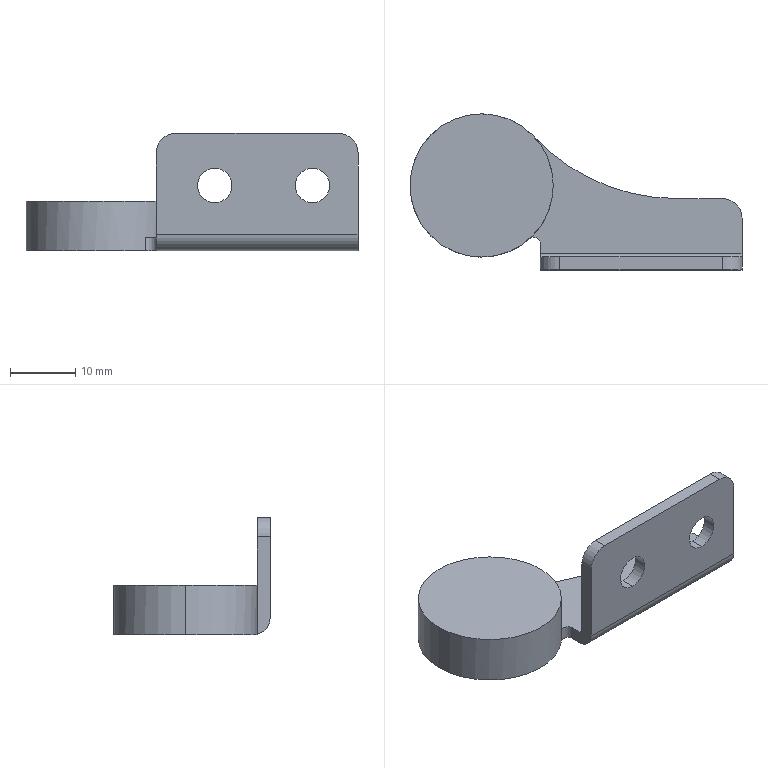Part | SolidWorks | features BaseBody 1 | 1 solid | 42 faces | box 51 x 24 x 18 mm | volume 4459 mm3 | cylinder 25 | plane 17 | commonest cylinder face diameters 0.528 x8 5.3 x4 6 x3 10 x2 10.02 x2 22 x2
STEP:
#1=CARTESIAN_POINT('',(-11.,0.,3.5));
#2=VERTEX_POINT('',#1);
#3=CARTESIAN_POINT('',(8.035,7.512,3.5));
#4=VERTEX_POINT('',#3);
#5=CARTESIAN_POINT('',(0.,0.,3.5));
#6=DIRECTION('',(0.,0.,-1.));
#7=DIRECTION('',(1.,0.,0.));
#8=AXIS2_PLACEMENT_3D('',#5,#6,#7);
#9=CIRCLE('',#8,11.);
#10=EDGE_CURVE('',#2,#4,#9,.T.);
#11=ORIENTED_EDGE('',*,*,#10,.F.);
#12=CARTESIAN_POINT('',(-11.,0.,11.1));
#13=VERTEX_POINT('',#12);
#14=CARTESIAN_POINT('',(-11.,0.,60.062));
#15=DIRECTION('',(0.,0.,1.));
#16=VECTOR('',#15,1000.);
#17=LINE('',#14,#16);
#18=EDGE_CURVE('',#2,#13,#17,.T.);
#19=ORIENTED_EDGE('',*,*,#18,.T.);
#20=CARTESIAN_POINT('',(11.,0.,11.1));
#21=VERTEX_POINT('',#20);
#22=CARTESIAN_POINT('',(0.,0.,11.1));
#23=DIRECTION('',(0.,0.,-1.));
#24=DIRECTION('',(1.,0.,0.));
#25=AXIS2_PLACEMENT_3D('',#22,#23,#24);
#26=CIRCLE('',#25,11.);
#27=EDGE_CURVE('',#13,#21,#26,.T.);
#28=ORIENTED_EDGE('',*,*,#27,.T.);
#29=CARTESIAN_POINT('',(11.,0.,5.5));
#30=VERTEX_POINT('',#29);
#31=CARTESIAN_POINT('',(11.,0.,60.062));
#32=DIRECTION('',(0.,0.,1.));
#33=VECTOR('',#32,1000.);
#34=LINE('',#31,#33);
#35=EDGE_CURVE('',#30,#21,#34,.T.);
#36=ORIENTED_EDGE('',*,*,#35,.F.);
#37=CARTESIAN_POINT('',(8.035,7.512,5.5));
#38=VERTEX_POINT('',#37);
#39=CARTESIAN_POINT('',(0.,0.,5.5));
#40=DIRECTION('',(0.,0.,1.));
#41=DIRECTION('',(1.,0.,0.));
#42=AXIS2_PLACEMENT_3D('',#39,#40,#41);
#43=CIRCLE('',#42,11.);
#44=EDGE_CURVE('',#30,#38,#43,.T.);
#45=ORIENTED_EDGE('',*,*,#44,.T.);
#46=CARTESIAN_POINT('',(8.035,7.512,3.5));
#47=DIRECTION('',(0.,0.,-1.));
#48=VECTOR('',#47,1000.);
#49=LINE('',#46,#48);
#50=EDGE_CURVE('',#38,#4,#49,.T.);
#51=ORIENTED_EDGE('',*,*,#50,.T.);
#52=EDGE_LOOP('',(#11,#19,#28,#36,#45,#51));
#53=FACE_OUTER_BOUND('',#52,.T.);
#54=CARTESIAN_POINT('',(0.,0.,60.062));
#55=DIRECTION('',(0.,0.,1.));
#56=DIRECTION('',(1.,0.,0.));
#57=AXIS2_PLACEMENT_3D('',#54,#55,#56);
#58=CYLINDRICAL_SURFACE('',#57,11.);
#59=ADVANCED_FACE('',(#53),#58,.T.);
#60=CARTESIAN_POINT('',(5.,0.,3.5));
#61=VERTEX_POINT('',#60);
#62=CARTESIAN_POINT('',(-5.,0.,3.5));
#63=VERTEX_POINT('',#62);
#64=CARTESIAN_POINT('',(0.,0.,3.5));
#65=DIRECTION('',(0.,0.,1.));
#66=DIRECTION('',(1.,0.,0.));
#67=AXIS2_PLACEMENT_3D('',#64,#65,#66);
#68=CIRCLE('',#67,5.);
#69=EDGE_CURVE('',#61,#63,#68,.T.);
#70=ORIENTED_EDGE('',*,*,#69,.T.);
#71=CARTESIAN_POINT('',(-5.,0.,5.5));
#72=VERTEX_POINT('',#71);
#73=CARTESIAN_POINT('',(-5.,0.,60.062));
#74=DIRECTION('',(0.,0.,1.));
#75=VECTOR('',#74,1000.);
#76=LINE('',#73,#75);
#77=EDGE_CURVE('',#63,#72,#76,.T.);
#78=ORIENTED_EDGE('',*,*,#77,.T.);
#79=CARTESIAN_POINT('',(5.,0.,5.5));
#80=VERTEX_POINT('',#79);
#81=CARTESIAN_POINT('',(0.,0.,5.5));
#82=DIRECTION('',(0.,0.,1.));
#83=DIRECTION('',(1.,0.,0.));
#84=AXIS2_PLACEMENT_3D('',#81,#82,#83);
#85=CIRCLE('',#84,5.);
#86=EDGE_CURVE('',#80,#72,#85,.T.);
#87=ORIENTED_EDGE('',*,*,#86,.F.);
#88=CARTESIAN_POINT('',(5.,0.,60.062));
#89=DIRECTION('',(0.,0.,1.));
#90=VECTOR('',#89,1000.);
#91=LINE('',#88,#90);
#92=EDGE_CURVE('',#61,#80,#91,.T.);
#93=ORIENTED_EDGE('',*,*,#92,.F.);
#94=EDGE_LOOP('',(#70,#78,#87,#93));
#95=FACE_OUTER_BOUND('',#94,.T.);
#96=CARTESIAN_POINT('',(0.,0.,60.062));
#97=DIRECTION('',(0.,0.,1.));
#98=DIRECTION('',(1.,0.,0.));
#99=AXIS2_PLACEMENT_3D('',#96,#97,#98);
#100=CYLINDRICAL_SURFACE('',#99,5.);
#101=ADVANCED_FACE('',(#95),#100,.T.);
#102=CARTESIAN_POINT('',(18.,-13.,16.15));
#103=VERTEX_POINT('',#102);
#104=CARTESIAN_POINT('',(18.,-13.,10.85));
#105=VERTEX_POINT('',#104);
#106=CARTESIAN_POINT('',(18.,-13.,13.5));
#107=DIRECTION('',(0.,-1.,0.));
#108=DIRECTION('',(0.,0.,1.));
#109=AXIS2_PLACEMENT_3D('',#106,#107,#108);
#110=CIRCLE('',#109,2.65);
#111=EDGE_CURVE('',#103,#105,#110,.T.);
#112=ORIENTED_EDGE('',*,*,#111,.T.);
#113=CARTESIAN_POINT('',(18.,-11.,10.85));
#114=VERTEX_POINT('',#113);
#115=CARTESIAN_POINT('',(18.,-13.,10.85));
#116=DIRECTION('',(0.,1.,0.));
#117=VECTOR('',#116,1000.);
#118=LINE('',#115,#117);
#119=EDGE_CURVE('',#105,#114,#118,.T.);
#120=ORIENTED_EDGE('',*,*,#119,.T.);
#121=CARTESIAN_POINT('',(18.,-11.,16.15));
#122=VERTEX_POINT('',#121);
#123=CARTESIAN_POINT('',(18.,-11.,13.5));
#124=DIRECTION('',(0.,-1.,0.));
#125=DIRECTION('',(0.,0.,1.));
#126=AXIS2_PLACEMENT_3D('',#123,#124,#125);
#127=CIRCLE('',#126,2.65);
#128=EDGE_CURVE('',#122,#114,#127,.T.);
#129=ORIENTED_EDGE('',*,*,#128,.F.);
#130=CARTESIAN_POINT('',(18.,-13.,16.15));
#131=DIRECTION('',(0.,1.,0.));
#132=VECTOR('',#131,1000.);
#133=LINE('',#130,#132);
#134=EDGE_CURVE('',#103,#122,#133,.T.);
#135=ORIENTED_EDGE('',*,*,#134,.F.);
#136=EDGE_LOOP('',(#112,#120,#129,#135));
#137=FACE_OUTER_BOUND('',#136,.T.);
#138=CARTESIAN_POINT('',(18.,-13.,13.5));
#139=DIRECTION('',(0.,1.,0.));
#140=DIRECTION('',(0.,0.,1.));
#141=AXIS2_PLACEMENT_3D('',#138,#139,#140);
#142=CYLINDRICAL_SURFACE('',#141,2.65);
#143=ADVANCED_FACE('',(#137),#142,.F.);
#144=CARTESIAN_POINT('',(33.,-13.,16.15));
#145=VERTEX_POINT('',#144);
#146=CARTESIAN_POINT('',(33.,-13.,10.85));
#147=VERTEX_POINT('',#146);
#148=CARTESIAN_POINT('',(33.,-13.,13.5));
#149=DIRECTION('',(0.,-1.,0.));
#150=DIRECTION('',(0.,0.,1.));
#151=AXIS2_PLACEMENT_3D('',#148,#149,#150);
#152=CIRCLE('',#151,2.65);
#153=EDGE_CURVE('',#145,#147,#152,.T.);
#154=ORIENTED_EDGE('',*,*,#153,.T.);
#155=CARTESIAN_POINT('',(33.,-11.,10.85));
#156=VERTEX_POINT('',#155);
#157=CARTESIAN_POINT('',(33.,-13.,10.85));
#158=DIRECTION('',(0.,1.,0.));
#159=VECTOR('',#158,1000.);
#160=LINE('',#157,#159);
#161=EDGE_CURVE('',#147,#156,#160,.T.);
#162=ORIENTED_EDGE('',*,*,#161,.T.);
#163=CARTESIAN_POINT('',(33.,-11.,16.15));
#164=VERTEX_POINT('',#163);
#165=CARTESIAN_POINT('',(33.,-11.,13.5));
#166=DIRECTION('',(0.,-1.,0.));
#167=DIRECTION('',(0.,0.,1.));
#168=AXIS2_PLACEMENT_3D('',#165,#166,#167);
#169=CIRCLE('',#168,2.65);
#170=EDGE_CURVE('',#164,#156,#169,.T.);
#171=ORIENTED_EDGE('',*,*,#170,.F.);
#172=CARTESIAN_POINT('',(33.,-13.,16.15));
#173=DIRECTION('',(0.,1.,0.));
#174=VECTOR('',#173,1000.);
#175=LINE('',#172,#174);
#176=EDGE_CURVE('',#145,#164,#175,.T.);
#177=ORIENTED_EDGE('',*,*,#176,.F.);
#178=EDGE_LOOP('',(#154,#162,#171,#177));
#179=FACE_OUTER_BOUND('',#178,.T.);
#180=CARTESIAN_POINT('',(33.,-13.,13.5));
#181=DIRECTION('',(0.,1.,0.));
#182=DIRECTION('',(0.,0.,1.));
#183=AXIS2_PLACEMENT_3D('',#180,#181,#182);
#184=CYLINDRICAL_SURFACE('',#183,2.65);
#185=ADVANCED_FACE('',(#179),#184,.F.);
#186=CARTESIAN_POINT('',(4.321,-2.76,3.5));
#187=VERTEX_POINT('',#186);
#188=CARTESIAN_POINT('',(4.105,-2.873,3.5));
#189=VERTEX_POINT('',#188);
#190=CARTESIAN_POINT('',(4.321,-3.024,3.5));
#191=DIRECTION('',(0.,0.,1.));
#192=DIRECTION('',(1.,0.,0.));
#193=AXIS2_PLACEMENT_3D('',#190,#191,#192);
#194=CIRCLE('',#193,0.264);
#195=EDGE_CURVE('',#187,#189,#194,.T.);
#196=ORIENTED_EDGE('',*,*,#195,.F.);
#197=CARTESIAN_POINT('',(6.436,-2.76,3.5));
#198=VERTEX_POINT('',#197);
#199=CARTESIAN_POINT('',(29.95,-2.76,3.5));
#200=DIRECTION('',(1.,0.,0.));
#201=VECTOR('',#200,1000.);
#202=LINE('',#199,#201);
#203=EDGE_CURVE('',#187,#198,#202,.T.);
#204=ORIENTED_EDGE('',*,*,#203,.T.);
#205=CARTESIAN_POINT('',(6.7,-2.496,3.5));
#206=VERTEX_POINT('',#205);
#207=CARTESIAN_POINT('',(6.436,-2.496,3.5));
#208=DIRECTION('',(0.,0.,1.));
#209=DIRECTION('',(1.,0.,0.));
#210=AXIS2_PLACEMENT_3D('',#207,#208,#209);
#211=CIRCLE('',#210,0.264);
#212=EDGE_CURVE('',#198,#206,#211,.T.);
#213=ORIENTED_EDGE('',*,*,#212,.T.);
#214=CARTESIAN_POINT('',(6.7,2.496,3.5));
#215=VERTEX_POINT('',#214);
#216=CARTESIAN_POINT('',(6.7,28.,3.5));
#217=DIRECTION('',(0.,1.,0.));
#218=VECTOR('',#217,1000.);
#219=LINE('',#216,#218);
#220=EDGE_CURVE('',#206,#215,#219,.T.);
#221=ORIENTED_EDGE('',*,*,#220,.T.);
#222=CARTESIAN_POINT('',(6.436,2.76,3.5));
#223=VERTEX_POINT('',#222);
#224=CARTESIAN_POINT('',(6.436,2.496,3.5));
#225=DIRECTION('',(0.,0.,1.));
#226=DIRECTION('',(1.,0.,0.));
#227=AXIS2_PLACEMENT_3D('',#224,#225,#226);
#228=CIRCLE('',#227,0.264);
#229=EDGE_CURVE('',#215,#223,#228,.T.);
#230=ORIENTED_EDGE('',*,*,#229,.T.);
#231=CARTESIAN_POINT('',(4.321,2.76,3.5));
#232=VERTEX_POINT('',#231);
#233=CARTESIAN_POINT('',(29.95,2.76,3.5));
#234=DIRECTION('',(-1.,0.,0.));
#235=VECTOR('',#234,1000.);
#236=LINE('',#233,#235);
#237=EDGE_CURVE('',#223,#232,#236,.T.);
#238=ORIENTED_EDGE('',*,*,#237,.T.);
#239=CARTESIAN_POINT('',(4.105,2.873,3.5));
#240=VERTEX_POINT('',#239);
#241=CARTESIAN_POINT('',(4.321,3.024,3.5));
#242=DIRECTION('',(0.,0.,1.));
#243=DIRECTION('',(1.,0.,0.));
#244=AXIS2_PLACEMENT_3D('',#241,#242,#243);
#245=CIRCLE('',#244,0.264);
#246=EDGE_CURVE('',#240,#232,#245,.T.);
#247=ORIENTED_EDGE('',*,*,#246,.F.);
#248=CARTESIAN_POINT('',(-4.105,2.873,3.5));
#249=VERTEX_POINT('',#248);
#250=CARTESIAN_POINT('',(0.,0.,3.5));
#251=DIRECTION('',(0.,0.,1.));
#252=DIRECTION('',(1.,0.,0.));
#253=AXIS2_PLACEMENT_3D('',#250,#251,#252);
#254=CIRCLE('',#253,5.01);
#255=EDGE_CURVE('',#240,#249,#254,.T.);
#256=ORIENTED_EDGE('',*,*,#255,.T.);
#257=CARTESIAN_POINT('',(-4.321,2.76,3.5));
#258=VERTEX_POINT('',#257);
#259=CARTESIAN_POINT('',(-4.321,3.024,3.5));
#260=DIRECTION('',(0.,0.,1.));
#261=DIRECTION('',(1.,0.,0.));
#262=AXIS2_PLACEMENT_3D('',#259,#260,#261);
#263=CIRCLE('',#262,0.264);
#264=EDGE_CURVE('',#258,#249,#263,.T.);
#265=ORIENTED_EDGE('',*,*,#264,.F.);
#266=CARTESIAN_POINT('',(-6.436,2.76,3.5));
#267=VERTEX_POINT('',#266);
#268=CARTESIAN_POINT('',(29.95,2.76,3.5));
#269=DIRECTION('',(-1.,0.,0.));
#270=VECTOR('',#269,1000.);
#271=LINE('',#268,#270);
#272=EDGE_CURVE('',#258,#267,#271,.T.);
#273=ORIENTED_EDGE('',*,*,#272,.T.);
#274=CARTESIAN_POINT('',(-6.7,2.496,3.5));
#275=VERTEX_POINT('',#274);
#276=CARTESIAN_POINT('',(-6.436,2.496,3.5));
#277=DIRECTION('',(0.,0.,1.));
#278=DIRECTION('',(1.,0.,0.));
#279=AXIS2_PLACEMENT_3D('',#276,#277,#278);
#280=CIRCLE('',#279,0.264);
#281=EDGE_CURVE('',#267,#275,#280,.T.);
#282=ORIENTED_EDGE('',*,*,#281,.T.);
#283=CARTESIAN_POINT('',(-6.7,-2.496,3.5));
#284=VERTEX_POINT('',#283);
#285=CARTESIAN_POINT('',(-6.7,28.,3.5));
#286=DIRECTION('',(0.,-1.,0.));
#287=VECTOR('',#286,1000.);
#288=LINE('',#285,#287);
#289=EDGE_CURVE('',#275,#284,#288,.T.);
#290=ORIENTED_EDGE('',*,*,#289,.T.);
#291=CARTESIAN_POINT('',(-6.436,-2.76,3.5));
#292=VERTEX_POINT('',#291);
#293=CARTESIAN_POINT('',(-6.436,-2.496,3.5));
#294=DIRECTION('',(0.,0.,1.));
#295=DIRECTION('',(1.,0.,0.));
#296=AXIS2_PLACEMENT_3D('',#293,#294,#295);
#297=CIRCLE('',#296,0.264);
#298=EDGE_CURVE('',#284,#292,#297,.T.);
#299=ORIENTED_EDGE('',*,*,#298,.T.);
#300=CARTESIAN_POINT('',(-4.321,-2.76,3.5));
#301=VERTEX_POINT('',#300);
#302=CARTESIAN_POINT('',(29.95,-2.76,3.5));
#303=DIRECTION('',(1.,0.,0.));
#304=VECTOR('',#303,1000.);
#305=LINE('',#302,#304);
#306=EDGE_CURVE('',#292,#301,#305,.T.);
#307=ORIENTED_EDGE('',*,*,#306,.T.);
#308=CARTESIAN_POINT('',(-4.105,-2.873,3.5));
#309=VERTEX_POINT('',#308);
#310=CARTESIAN_POINT('',(-4.321,-3.024,3.5));
#311=DIRECTION('',(0.,0.,1.));
#312=DIRECTION('',(1.,0.,0.));
#313=AXIS2_PLACEMENT_3D('',#310,#311,#312);
#314=CIRCLE('',#313,0.264);
#315=EDGE_CURVE('',#309,#301,#314,.T.);
#316=ORIENTED_EDGE('',*,*,#315,.F.);
#317=CARTESIAN_POINT('',(0.,0.,3.5));
#318=DIRECTION('',(0.,0.,1.));
#319=DIRECTION('',(1.,0.,0.));
#320=AXIS2_PLACEMENT_3D('',#317,#318,#319);
#321=CIRCLE('',#320,5.01);
#322=EDGE_CURVE('',#309,#189,#321,.T.);
#323=ORIENTED_EDGE('',*,*,#322,.T.);
#324=EDGE_LOOP('',(#196,#204,#213,#221,#230,#238,#247,#256,#265,#273,#282,#290,#299,#307,#316,#323));
#325=FACE_BOUND('',#324,.T.);
#326=CARTESIAN_POINT('',(29.95,-2.,3.5));
#327=VERTEX_POINT('',#326);
#328=CARTESIAN_POINT('',(37.,-2.,3.5));
#329=VERTEX_POINT('',#328);
#330=CARTESIAN_POINT('',(29.95,-2.,3.5));
#331=DIRECTION('',(1.,0.,0.));
#332=VECTOR('',#331,1000.);
#333=LINE('',#330,#332);
#334=EDGE_CURVE('',#327,#329,#333,.T.);
#335=ORIENTED_EDGE('',*,*,#334,.T.);
#336=CARTESIAN_POINT('',(40.,-5.,3.5));
#337=VERTEX_POINT('',#336);
#338=CARTESIAN_POINT('',(37.,-5.,3.5));
#339=DIRECTION('',(0.,0.,-1.));
#340=DIRECTION('',(1.,0.,0.));
#341=AXIS2_PLACEMENT_3D('',#338,#339,#340);
#342=CIRCLE('',#341,3.);
#343=EDGE_CURVE('',#329,#337,#342,.T.);
#344=ORIENTED_EDGE('',*,*,#343,.T.);
#345=CARTESIAN_POINT('',(40.,-10.5,3.5));
#346=VERTEX_POINT('',#345);
#347=CARTESIAN_POINT('',(40.,28.,3.5));
#348=DIRECTION('',(0.,-1.,0.));
#349=VECTOR('',#348,1000.);
#350=LINE('',#347,#349);
#351=EDGE_CURVE('',#337,#346,#350,.T.);
#352=ORIENTED_EDGE('',*,*,#351,.T.);
#353=CARTESIAN_POINT('',(9.,-10.5,3.5));
#354=VERTEX_POINT('',#353);
#355=CARTESIAN_POINT('',(29.95,-10.5,3.5));
#356=DIRECTION('',(-1.,0.,0.));
#357=VECTOR('',#356,1000.);
#358=LINE('',#355,#357);
#359=EDGE_CURVE('',#346,#354,#358,.T.);
#360=ORIENTED_EDGE('',*,*,#359,.T.);
#361=CARTESIAN_POINT('',(9.,-8.944,3.5));
#362=VERTEX_POINT('',#361);
#363=CARTESIAN_POINT('',(9.,-13.,3.5));
#364=DIRECTION('',(0.,-1.,0.));
#365=VECTOR('',#364,1000.);
#366=LINE('',#363,#365);
#367=EDGE_CURVE('',#362,#354,#366,.T.);
#368=ORIENTED_EDGE('',*,*,#367,.F.);
#369=CARTESIAN_POINT('',(7.333,-8.199,3.5));
#370=VERTEX_POINT('',#369);
#371=CARTESIAN_POINT('',(8.,-8.944,3.5));
#372=DIRECTION('',(0.,0.,1.));
#373=DIRECTION('',(1.,0.,0.));
#374=AXIS2_PLACEMENT_3D('',#371,#372,#373);
#375=CIRCLE('',#374,1.);
#376=EDGE_CURVE('',#362,#370,#375,.T.);
#377=ORIENTED_EDGE('',*,*,#376,.T.);
#378=CARTESIAN_POINT('',(0.,0.,3.5));
#379=DIRECTION('',(0.,0.,-1.));
#380=DIRECTION('',(1.,0.,0.));
#381=AXIS2_PLACEMENT_3D('',#378,#379,#380);
#382=CIRCLE('',#381,11.);
#383=EDGE_CURVE('',#370,#2,#382,.T.);
#384=ORIENTED_EDGE('',*,*,#383,.T.);
#385=ORIENTED_EDGE('',*,*,#10,.T.);
#386=CARTESIAN_POINT('',(29.95,28.,3.5));
#387=DIRECTION('',(0.,0.,1.));
#388=DIRECTION('',(1.,0.,0.));
#389=AXIS2_PLACEMENT_3D('',#386,#387,#388);
#390=CIRCLE('',#389,30.);
#391=EDGE_CURVE('',#4,#327,#390,.T.);
#392=ORIENTED_EDGE('',*,*,#391,.T.);
#393=EDGE_LOOP('',(#335,#344,#352,#360,#368,#377,#384,#385,#392));
#394=FACE_OUTER_BOUND('',#393,.T.);
#395=CARTESIAN_POINT('',(29.95,28.,3.5));
#396=DIRECTION('',(0.,0.,-1.));
#397=DIRECTION('',(-1.,0.,0.));
#398=AXIS2_PLACEMENT_3D('',#395,#396,#397);
#399=PLANE('',#398);
#400=ADVANCED_FACE('',(#325,#394),#399,.T.);
#401=CARTESIAN_POINT('',(6.436,-2.76,5.5));
#402=VERTEX_POINT('',#401);
#403=CARTESIAN_POINT('',(6.436,-2.76,3.5));
#404=DIRECTION('',(0.,0.,1.));
#405=VECTOR('',#404,1000.);
#406=LINE('',#403,#405);
#407=EDGE_CURVE('',#198,#402,#406,.T.);
#408=ORIENTED_EDGE('',*,*,#407,.F.);
#409=ORIENTED_EDGE('',*,*,#203,.F.);
#410=CARTESIAN_POINT('',(4.321,-2.76,5.5));
#411=VERTEX_POINT('',#410);
#412=CARTESIAN_POINT('',(4.321,-2.76,3.5));
#413=DIRECTION('',(0.,0.,-1.));
#414=VECTOR('',#413,1000.);
#415=LINE('',#412,#414);
#416=EDGE_CURVE('',#411,#187,#415,.T.);
#417=ORIENTED_EDGE('',*,*,#416,.F.);
#418=CARTESIAN_POINT('',(4.321,-2.76,5.5));
#419=DIRECTION('',(-1.,0.,0.));
#420=VECTOR('',#419,1000.);
#421=LINE('',#418,#420);
#422=EDGE_CURVE('',#402,#411,#421,.T.);
#423=ORIENTED_EDGE('',*,*,#422,.F.);
#424=EDGE_LOOP('',(#408,#409,#417,#423));
#425=FACE_OUTER_BOUND('',#424,.T.);
#426=CARTESIAN_POINT('',(4.321,-2.76,3.5));
#427=DIRECTION('',(0.,-1.,0.));
#428=DIRECTION('',(0.,0.,-1.));
#429=AXIS2_PLACEMENT_3D('',#426,#427,#428);
#430=PLANE('',#429);
#431=ADVANCED_FACE('',(#425),#430,.F.);
#432=CARTESIAN_POINT('',(4.105,-2.873,5.5));
#433=VERTEX_POINT('',#432);
#434=CARTESIAN_POINT('',(4.105,-2.873,3.5));
#435=DIRECTION('',(0.,0.,1.));
#436=VECTOR('',#435,1000.);
#437=LINE('',#434,#436);
#438=EDGE_CURVE('',#189,#433,#437,.T.);
#439=ORIENTED_EDGE('',*,*,#438,.F.);
#440=ORIENTED_EDGE('',*,*,#322,.F.);
#441=CARTESIAN_POINT('',(-4.105,-2.873,5.5));
#442=VERTEX_POINT('',#441);
#443=CARTESIAN_POINT('',(-4.105,-2.873,3.5));
#444=DIRECTION('',(0.,0.,-1.));
#445=VECTOR('',#444,1000.);
#446=LINE('',#443,#445);
#447=EDGE_CURVE('',#442,#309,#446,.T.);
#448=ORIENTED_EDGE('',*,*,#447,.F.);
#449=CARTESIAN_POINT('',(0.,0.,5.5));
#450=DIRECTION('',(0.,0.,-1.));
#451=DIRECTION('',(1.,0.,0.));
#452=AXIS2_PLACEMENT_3D('',#449,#450,#451);
#453=CIRCLE('',#452,5.01);
#454=EDGE_CURVE('',#433,#442,#453,.T.);
#455=ORIENTED_EDGE('',*,*,#454,.F.);
#456=EDGE_LOOP('',(#439,#440,#448,#455));
#457=FACE_OUTER_BOUND('',#456,.T.);
#458=CARTESIAN_POINT('',(0.,0.,3.5));
#459=DIRECTION('',(0.,0.,1.));
#460=DIRECTION('',(1.,0.,0.));
#461=AXIS2_PLACEMENT_3D('',#458,#459,#460);
#462=CYLINDRICAL_SURFACE('',#461,5.01);
#463=ADVANCED_FACE('',(#457),#462,.F.);
#464=CARTESIAN_POINT('',(-4.321,-2.76,5.5));
#465=VERTEX_POINT('',#464);
#466=CARTESIAN_POINT('',(-4.321,-2.76,3.5));
#467=DIRECTION('',(0.,0.,1.));
#468=VECTOR('',#467,1000.);
#469=LINE('',#466,#468);
#470=EDGE_CURVE('',#301,#465,#469,.T.);
#471=ORIENTED_EDGE('',*,*,#470,.F.);
#472=ORIENTED_EDGE('',*,*,#306,.F.);
#473=CARTESIAN_POINT('',(-6.436,-2.76,5.5));
#474=VERTEX_POINT('',#473);
#475=CARTESIAN_POINT('',(-6.436,-2.76,3.5));
#476=DIRECTION('',(0.,0.,-1.));
#477=VECTOR('',#476,1000.);
#478=LINE('',#475,#477);
#479=EDGE_CURVE('',#474,#292,#478,.T.);
#480=ORIENTED_EDGE('',*,*,#479,.F.);
#481=CARTESIAN_POINT('',(-6.436,-2.76,5.5));
#482=DIRECTION('',(-1.,0.,0.));
#483=VECTOR('',#482,1000.);
#484=LINE('',#481,#483);
#485=EDGE_CURVE('',#465,#474,#484,.T.);
#486=ORIENTED_EDGE('',*,*,#485,.F.);
#487=EDGE_LOOP('',(#471,#472,#480,#486));
#488=FACE_OUTER_BOUND('',#487,.T.);
#489=CARTESIAN_POINT('',(-6.436,-2.76,3.5));
#490=DIRECTION('',(0.,-1.,0.));
#491=DIRECTION('',(0.,0.,-1.));
#492=AXIS2_PLACEMENT_3D('',#489,#490,#491);
#493=PLANE('',#492);
#494=ADVANCED_FACE('',(#488),#493,.F.);
#495=CARTESIAN_POINT('',(-6.7,-2.496,5.5));
#496=VERTEX_POINT('',#495);
#497=CARTESIAN_POINT('',(-6.7,-2.496,3.5));
#498=DIRECTION('',(0.,0.,1.));
#499=VECTOR('',#498,1000.);
#500=LINE('',#497,#499);
#501=EDGE_CURVE('',#284,#496,#500,.T.);
#502=ORIENTED_EDGE('',*,*,#501,.F.);
#503=ORIENTED_EDGE('',*,*,#289,.F.);
#504=CARTESIAN_POINT('',(-6.7,2.496,5.5));
#505=VERTEX_POINT('',#504);
#506=CARTESIAN_POINT('',(-6.7,2.496,3.5));
#507=DIRECTION('',(0.,0.,-1.));
#508=VECTOR('',#507,1000.);
#509=LINE('',#506,#508);
#510=EDGE_CURVE('',#505,#275,#509,.T.);
#511=ORIENTED_EDGE('',*,*,#510,.F.);
#512=CARTESIAN_POINT('',(-6.7,2.496,5.5));
#513=DIRECTION('',(0.,1.,0.));
#514=VECTOR('',#513,1000.);
#515=LINE('',#512,#514);
#516=EDGE_CURVE('',#496,#505,#515,.T.);
#517=ORIENTED_EDGE('',*,*,#516,.F.);
#518=EDGE_LOOP('',(#502,#503,#511,#517));
#519=FACE_OUTER_BOUND('',#518,.T.);
#520=CARTESIAN_POINT('',(-6.7,2.496,3.5));
#521=DIRECTION('',(-1.,0.,0.));
#522=DIRECTION('',(0.,-1.,0.));
#523=AXIS2_PLACEMENT_3D('',#520,#521,#522);
#524=PLANE('',#523);
#525=ADVANCED_FACE('',(#519),#524,.F.);
#526=CARTESIAN_POINT('',(-6.436,2.76,5.5));
#527=VERTEX_POINT('',#526);
#528=CARTESIAN_POINT('',(-6.436,2.76,3.5));
#529=DIRECTION('',(0.,0.,1.));
#530=VECTOR('',#529,1000.);
#531=LINE('',#528,#530);
#532=EDGE_CURVE('',#267,#527,#531,.T.);
#533=ORIENTED_EDGE('',*,*,#532,.F.);
#534=ORIENTED_EDGE('',*,*,#272,.F.);
#535=CARTESIAN_POINT('',(-4.321,2.76,5.5));
#536=VERTEX_POINT('',#535);
#537=CARTESIAN_POINT('',(-4.321,2.76,3.5));
#538=DIRECTION('',(0.,0.,-1.));
#539=VECTOR('',#538,1000.);
#540=LINE('',#537,#539);
#541=EDGE_CURVE('',#536,#258,#540,.T.);
#542=ORIENTED_EDGE('',*,*,#541,.F.);
#543=CARTESIAN_POINT('',(-6.436,2.76,5.5));
#544=DIRECTION('',(1.,0.,0.));
#545=VECTOR('',#544,1000.);
#546=LINE('',#543,#545);
#547=EDGE_CURVE('',#527,#536,#546,.T.);
#548=ORIENTED_EDGE('',*,*,#547,.F.);
#549=EDGE_LOOP('',(#533,#534,#542,#548));
#550=FACE_OUTER_BOUND('',#549,.T.);
#551=CARTESIAN_POINT('',(-6.436,2.76,3.5));
#552=DIRECTION('',(0.,1.,0.));
#553=DIRECTION('',(0.,0.,1.));
#554=AXIS2_PLACEMENT_3D('',#551,#552,#553);
#555=PLANE('',#554);
#556=ADVANCED_FACE('',(#550),#555,.F.);
#557=CARTESIAN_POINT('',(-4.105,2.873,5.5));
#558=VERTEX_POINT('',#557);
#559=CARTESIAN_POINT('',(-4.105,2.873,3.5));
#560=DIRECTION('',(0.,0.,1.));
#561=VECTOR('',#560,1000.);
#562=LINE('',#559,#561);
#563=EDGE_CURVE('',#249,#558,#562,.T.);
#564=ORIENTED_EDGE('',*,*,#563,.F.);
#565=ORIENTED_EDGE('',*,*,#255,.F.);
#566=CARTESIAN_POINT('',(4.105,2.873,5.5));
#567=VERTEX_POINT('',#566);
#568=CARTESIAN_POINT('',(4.105,2.873,3.5));
#569=DIRECTION('',(0.,0.,-1.));
#570=VECTOR('',#569,1000.);
#571=LINE('',#568,#570);
#572=EDGE_CURVE('',#567,#240,#571,.T.);
#573=ORIENTED_EDGE('',*,*,#572,.F.);
#574=CARTESIAN_POINT('',(0.,0.,5.5));
#575=DIRECTION('',(0.,0.,-1.));
#576=DIRECTION('',(1.,0.,0.));
#577=AXIS2_PLACEMENT_3D('',#574,#575,#576);
#578=CIRCLE('',#577,5.01);
#579=EDGE_CURVE('',#558,#567,#578,.T.);
#580=ORIENTED_EDGE('',*,*,#579,.F.);
#581=EDGE_LOOP('',(#564,#565,#573,#580));
#582=FACE_OUTER_BOUND('',#581,.T.);
#583=CARTESIAN_POINT('',(0.,0.,3.5));
#584=DIRECTION('',(0.,0.,1.));
#585=DIRECTION('',(1.,0.,0.));
#586=AXIS2_PLACEMENT_3D('',#583,#584,#585);
#587=CYLINDRICAL_SURFACE('',#586,5.01);
#588=ADVANCED_FACE('',(#582),#587,.F.);
#589=CARTESIAN_POINT('',(4.321,2.76,5.5));
#590=VERTEX_POINT('',#589);
#591=CARTESIAN_POINT('',(4.321,2.76,3.5));
#592=DIRECTION('',(0.,0.,1.));
#593=VECTOR('',#592,1000.);
#594=LINE('',#591,#593);
#595=EDGE_CURVE('',#232,#590,#594,.T.);
#596=ORIENTED_EDGE('',*,*,#595,.F.);
#597=ORIENTED_EDGE('',*,*,#237,.F.);
#598=CARTESIAN_POINT('',(6.436,2.76,5.5));
#599=VERTEX_POINT('',#598);
#600=CARTESIAN_POINT('',(6.436,2.76,3.5));
#601=DIRECTION('',(0.,0.,-1.));
#602=VECTOR('',#601,1000.);
#603=LINE('',#600,#602);
#604=EDGE_CURVE('',#599,#223,#603,.T.);
#605=ORIENTED_EDGE('',*,*,#604,.F.);
#606=CARTESIAN_POINT('',(4.321,2.76,5.5));
#607=DIRECTION('',(1.,0.,0.));
#608=VECTOR('',#607,1000.);
#609=LINE('',#606,#608);
#610=EDGE_CURVE('',#590,#599,#609,.T.);
#611=ORIENTED_EDGE('',*,*,#610,.F.);
#612=EDGE_LOOP('',(#596,#597,#605,#611));
#613=FACE_OUTER_BOUND('',#612,.T.);
#614=CARTESIAN_POINT('',(4.321,2.76,3.5));
#615=DIRECTION('',(0.,1.,0.));
#616=DIRECTION('',(0.,0.,1.));
#617=AXIS2_PLACEMENT_3D('',#614,#615,#616);
#618=PLANE('',#617);
#619=ADVANCED_FACE('',(#613),#618,.F.);
#620=CARTESIAN_POINT('',(6.7,2.496,5.5));
#621=VERTEX_POINT('',#620);
#622=CARTESIAN_POINT('',(6.7,2.496,3.5));
#623=DIRECTION('',(0.,0.,1.));
#624=VECTOR('',#623,1000.);
#625=LINE('',#622,#624);
#626=EDGE_CURVE('',#215,#621,#625,.T.);
#627=ORIENTED_EDGE('',*,*,#626,.F.);
#628=ORIENTED_EDGE('',*,*,#220,.F.);
#629=CARTESIAN_POINT('',(6.7,-2.496,5.5));
#630=VERTEX_POINT('',#629);
#631=CARTESIAN_POINT('',(6.7,-2.496,3.5));
#632=DIRECTION('',(0.,0.,-1.));
#633=VECTOR('',#632,1000.);
#634=LINE('',#631,#633);
#635=EDGE_CURVE('',#630,#206,#634,.T.);
#636=ORIENTED_EDGE('',*,*,#635,.F.);
#637=CARTESIAN_POINT('',(6.7,2.496,5.5));
#638=DIRECTION('',(0.,-1.,0.));
#639=VECTOR('',#638,1000.);
#640=LINE('',#637,#639);
#641=EDGE_CURVE('',#621,#630,#640,.T.);
#642=ORIENTED_EDGE('',*,*,#641,.F.);
#643=EDGE_LOOP('',(#627,#628,#636,#642));
#644=FACE_OUTER_BOUND('',#643,.T.);
#645=CARTESIAN_POINT('',(6.7,2.496,3.5));
#646=DIRECTION('',(1.,0.,0.));
#647=DIRECTION('',(0.,0.,-1.));
#648=AXIS2_PLACEMENT_3D('',#645,#646,#647);
#649=PLANE('',#648);
#650=ADVANCED_FACE('',(#644),#649,.F.);
#651=ORIENTED_EDGE('',*,*,#343,.F.);
#652=CARTESIAN_POINT('',(37.,-2.,5.5));
#653=VERTEX_POINT('',#652);
#654=CARTESIAN_POINT('',(37.,-2.,3.5));
#655=DIRECTION('',(0.,0.,1.));
#656=VECTOR('',#655,1000.);
#657=LINE('',#654,#656);
#658=EDGE_CURVE('',#329,#653,#657,.T.);
#659=ORIENTED_EDGE('',*,*,#658,.T.);
#660=CARTESIAN_POINT('',(40.,-5.,5.5));
#661=VERTEX_POINT('',#660);
#662=CARTESIAN_POINT('',(37.,-5.,5.5));
#663=DIRECTION('',(0.,0.,-1.));
#664=DIRECTION('',(1.,0.,0.));
#665=AXIS2_PLACEMENT_3D('',#662,#663,#664);
#666=CIRCLE('',#665,3.);
#667=EDGE_CURVE('',#653,#661,#666,.T.);
#668=ORIENTED_EDGE('',*,*,#667,.T.);
#669=CARTESIAN_POINT('',(40.,-5.,3.5));
#670=DIRECTION('',(0.,0.,-1.));
#671=VECTOR('',#670,1000.);
#672=LINE('',#669,#671);
#673=EDGE_CURVE('',#661,#337,#672,.T.);
#674=ORIENTED_EDGE('',*,*,#673,.T.);
#675=EDGE_LOOP('',(#651,#659,#668,#674));
#676=FACE_OUTER_BOUND('',#675,.T.);
#677=CARTESIAN_POINT('',(37.,-5.,3.5));
#678=DIRECTION('',(0.,0.,1.));
#679=DIRECTION('',(1.,0.,0.));
#680=AXIS2_PLACEMENT_3D('',#677,#678,#679);
#681=CYLINDRICAL_SURFACE('',#680,3.);
#682=ADVANCED_FACE('',(#676),#681,.T.);
#683=ORIENTED_EDGE('',*,*,#334,.F.);
#684=CARTESIAN_POINT('',(29.95,-2.,5.5));
#685=VERTEX_POINT('',#684);
#686=CARTESIAN_POINT('',(29.95,-2.,3.5));
#687=DIRECTION('',(0.,0.,1.));
#688=VECTOR('',#687,1000.);
#689=LINE('',#686,#688);
#690=EDGE_CURVE('',#327,#685,#689,.T.);
#691=ORIENTED_EDGE('',*,*,#690,.T.);
#692=CARTESIAN_POINT('',(29.95,-2.,5.5));
#693=DIRECTION('',(1.,0.,0.));
#694=VECTOR('',#693,1000.);
#695=LINE('',#692,#694);
#696=EDGE_CURVE('',#685,#653,#695,.T.);
#697=ORIENTED_EDGE('',*,*,#696,.T.);
#698=ORIENTED_EDGE('',*,*,#658,.F.);
#699=EDGE_LOOP('',(#683,#691,#697,#698));
#700=FACE_OUTER_BOUND('',#699,.T.);
#701=CARTESIAN_POINT('',(29.95,-2.,3.5));
#702=DIRECTION('',(0.,1.,0.));
#703=DIRECTION('',(0.,0.,1.));
#704=AXIS2_PLACEMENT_3D('',#701,#702,#703);
#705=PLANE('',#704);
#706=ADVANCED_FACE('',(#700),#705,.T.);
#707=ORIENTED_EDGE('',*,*,#690,.F.);
#708=ORIENTED_EDGE('',*,*,#391,.F.);
#709=ORIENTED_EDGE('',*,*,#50,.F.);
#710=CARTESIAN_POINT('',(29.95,28.,5.5));
#711=DIRECTION('',(0.,0.,-1.));
#712=DIRECTION('',(1.,0.,0.));
#713=AXIS2_PLACEMENT_3D('',#710,#711,#712);
#714=CIRCLE('',#713,30.);
#715=EDGE_CURVE('',#685,#38,#714,.T.);
#716=ORIENTED_EDGE('',*,*,#715,.F.);
#717=EDGE_LOOP('',(#707,#708,#709,#716));
#718=FACE_OUTER_BOUND('',#717,.T.);
#719=CARTESIAN_POINT('',(29.95,28.,3.5));
#720=DIRECTION('',(0.,0.,1.));
#721=DIRECTION('',(1.,0.,0.));
#722=AXIS2_PLACEMENT_3D('',#719,#720,#721);
#723=CYLINDRICAL_SURFACE('',#722,30.);
#724=ADVANCED_FACE('',(#718),#723,.F.);
#725=ORIENTED_EDGE('',*,*,#18,.F.);
#726=ORIENTED_EDGE('',*,*,#383,.F.);
#727=CARTESIAN_POINT('',(7.333,-8.199,5.5));
#728=VERTEX_POINT('',#727);
#729=CARTESIAN_POINT('',(7.333,-8.199,60.062));
#730=DIRECTION('',(0.,0.,1.));
#731=VECTOR('',#730,1000.);
#732=LINE('',#729,#731);
#733=EDGE_CURVE('',#370,#728,#732,.T.);
#734=ORIENTED_EDGE('',*,*,#733,.T.);
#735=CARTESIAN_POINT('',(0.,0.,5.5));
#736=DIRECTION('',(0.,0.,1.));
#737=DIRECTION('',(1.,0.,0.));
#738=AXIS2_PLACEMENT_3D('',#735,#736,#737);
#739=CIRCLE('',#738,11.);
#740=EDGE_CURVE('',#728,#30,#739,.T.);
#741=ORIENTED_EDGE('',*,*,#740,.T.);
#742=ORIENTED_EDGE('',*,*,#35,.T.);
#743=CARTESIAN_POINT('',(0.,0.,11.1));
#744=DIRECTION('',(0.,0.,-1.));
#745=DIRECTION('',(1.,0.,0.));
#746=AXIS2_PLACEMENT_3D('',#743,#744,#745);
#747=CIRCLE('',#746,11.);
#748=EDGE_CURVE('',#21,#13,#747,.T.);
#749=ORIENTED_EDGE('',*,*,#748,.T.);
#750=EDGE_LOOP('',(#725,#726,#734,#741,#742,#749));
#751=FACE_OUTER_BOUND('',#750,.T.);
#752=CARTESIAN_POINT('',(0.,0.,60.062));
#753=DIRECTION('',(0.,0.,1.));
#754=DIRECTION('',(1.,0.,0.));
#755=AXIS2_PLACEMENT_3D('',#752,#753,#754);
#756=CYLINDRICAL_SURFACE('',#755,11.);
#757=ADVANCED_FACE('',(#751),#756,.T.);
#758=ORIENTED_EDGE('',*,*,#733,.F.);
#759=ORIENTED_EDGE('',*,*,#376,.F.);
#760=CARTESIAN_POINT('',(9.,-8.944,5.5));
#761=VERTEX_POINT('',#760);
#762=CARTESIAN_POINT('',(9.,-8.944,3.5));
#763=DIRECTION('',(0.,0.,-1.));
#764=VECTOR('',#763,1000.);
#765=LINE('',#762,#764);
#766=EDGE_CURVE('',#761,#362,#765,.T.);
#767=ORIENTED_EDGE('',*,*,#766,.F.);
#768=CARTESIAN_POINT('',(8.,-8.944,5.5));
#769=DIRECTION('',(0.,0.,-1.));
#770=DIRECTION('',(1.,0.,0.));
#771=AXIS2_PLACEMENT_3D('',#768,#769,#770);
#772=CIRCLE('',#771,1.);
#773=EDGE_CURVE('',#728,#761,#772,.T.);
#774=ORIENTED_EDGE('',*,*,#773,.F.);
#775=EDGE_LOOP('',(#758,#759,#767,#774));
#776=FACE_OUTER_BOUND('',#775,.T.);
#777=CARTESIAN_POINT('',(8.,-8.944,3.5));
#778=DIRECTION('',(0.,0.,1.));
#779=DIRECTION('',(1.,0.,0.));
#780=AXIS2_PLACEMENT_3D('',#777,#778,#779);
#781=CYLINDRICAL_SURFACE('',#780,1.);
#782=ADVANCED_FACE('',(#776),#781,.F.);
#783=CARTESIAN_POINT('',(40.,-13.,6.));
#784=VERTEX_POINT('',#783);
#785=CARTESIAN_POINT('',(9.,-13.,6.));
#786=VERTEX_POINT('',#785);
#787=CARTESIAN_POINT('',(40.,-13.,6.));
#788=DIRECTION('',(-1.,0.,0.));
#789=VECTOR('',#788,1000.);
#790=LINE('',#787,#789);
#791=EDGE_CURVE('',#784,#786,#790,.T.);
#792=ORIENTED_EDGE('',*,*,#791,.T.);
#793=CARTESIAN_POINT('',(9.,-10.5,6.));
#794=DIRECTION('',(1.,0.,0.));
#795=DIRECTION('',(0.,0.,-1.));
#796=AXIS2_PLACEMENT_3D('',#793,#794,#795);
#797=CIRCLE('',#796,2.5);
#798=EDGE_CURVE('',#786,#354,#797,.T.);
#799=ORIENTED_EDGE('',*,*,#798,.T.);
#800=ORIENTED_EDGE('',*,*,#359,.F.);
#801=CARTESIAN_POINT('',(40.,-10.5,6.));
#802=DIRECTION('',(-1.,0.,0.));
#803=DIRECTION('',(0.,0.,-1.));
#804=AXIS2_PLACEMENT_3D('',#801,#802,#803);
#805=CIRCLE('',#804,2.5);
#806=EDGE_CURVE('',#346,#784,#805,.T.);
#807=ORIENTED_EDGE('',*,*,#806,.T.);
#808=EDGE_LOOP('',(#792,#799,#800,#807));
#809=FACE_OUTER_BOUND('',#808,.T.);
#810=CARTESIAN_POINT('',(40.,-10.5,6.));
#811=DIRECTION('',(1.,0.,0.));
#812=DIRECTION('',(0.,0.,-1.));
#813=AXIS2_PLACEMENT_3D('',#810,#811,#812);
#814=CYLINDRICAL_SURFACE('',#813,2.5);
#815=ADVANCED_FACE('',(#809),#814,.T.);
#816=ORIENTED_EDGE('',*,*,#351,.F.);
#817=ORIENTED_EDGE('',*,*,#673,.F.);
#818=CARTESIAN_POINT('',(40.,-10.5,5.5));
#819=VERTEX_POINT('',#818);
#820=CARTESIAN_POINT('',(40.,-5.,5.5));
#821=DIRECTION('',(0.,-1.,0.));
#822=VECTOR('',#821,1000.);
#823=LINE('',#820,#822);
#824=EDGE_CURVE('',#661,#819,#823,.T.);
#825=ORIENTED_EDGE('',*,*,#824,.T.);
#826=CARTESIAN_POINT('',(40.,-11.,6.));
#827=VERTEX_POINT('',#826);
#828=CARTESIAN_POINT('',(40.,-10.5,6.));
#829=DIRECTION('',(1.,0.,0.));
#830=DIRECTION('',(0.,0.,-1.));
#831=AXIS2_PLACEMENT_3D('',#828,#829,#830);
#832=CIRCLE('',#831,0.5);
#833=EDGE_CURVE('',#827,#819,#832,.T.);
#834=ORIENTED_EDGE('',*,*,#833,.F.);
#835=CARTESIAN_POINT('',(40.,-11.,18.5));
#836=VERTEX_POINT('',#835);
#837=CARTESIAN_POINT('',(40.,-11.,18.5));
#838=DIRECTION('',(0.,0.,-1.));
#839=VECTOR('',#838,1000.);
#840=LINE('',#837,#839);
#841=EDGE_CURVE('',#836,#827,#840,.T.);
#842=ORIENTED_EDGE('',*,*,#841,.F.);
#843=CARTESIAN_POINT('',(40.,-13.,18.5));
#844=VERTEX_POINT('',#843);
#845=CARTESIAN_POINT('',(40.,-13.,18.5));
#846=DIRECTION('',(0.,1.,0.));
#847=VECTOR('',#846,1000.);
#848=LINE('',#845,#847);
#849=EDGE_CURVE('',#844,#836,#848,.T.);
#850=ORIENTED_EDGE('',*,*,#849,.F.);
#851=CARTESIAN_POINT('',(40.,-13.,18.5));
#852=DIRECTION('',(0.,0.,-1.));
#853=VECTOR('',#852,1000.);
#854=LINE('',#851,#853);
#855=EDGE_CURVE('',#844,#784,#854,.T.);
#856=ORIENTED_EDGE('',*,*,#855,.T.);
#857=ORIENTED_EDGE('',*,*,#806,.F.);
#858=EDGE_LOOP('',(#816,#817,#825,#834,#842,#850,#856,#857));
#859=FACE_OUTER_BOUND('',#858,.T.);
#860=CARTESIAN_POINT('',(40.,-5.,3.5));
#861=DIRECTION('',(1.,0.,0.));
#862=DIRECTION('',(0.,0.,-1.));
#863=AXIS2_PLACEMENT_3D('',#860,#861,#862);
#864=PLANE('',#863);
#865=ADVANCED_FACE('',(#859),#864,.T.);
#866=CARTESIAN_POINT('',(6.436,2.496,5.5));
#867=DIRECTION('',(0.,0.,-1.));
#868=DIRECTION('',(1.,0.,0.));
#869=AXIS2_PLACEMENT_3D('',#866,#867,#868);
#870=CIRCLE('',#869,0.264);
#871=EDGE_CURVE('',#599,#621,#870,.T.);
#872=ORIENTED_EDGE('',*,*,#871,.T.);
#873=ORIENTED_EDGE('',*,*,#641,.T.);
#874=CARTESIAN_POINT('',(6.436,-2.496,5.5));
#875=DIRECTION('',(0.,0.,-1.));
#876=DIRECTION('',(1.,0.,0.));
#877=AXIS2_PLACEMENT_3D('',#874,#875,#876);
#878=CIRCLE('',#877,0.264);
#879=EDGE_CURVE('',#630,#402,#878,.T.);
#880=ORIENTED_EDGE('',*,*,#879,.T.);
#881=ORIENTED_EDGE('',*,*,#422,.T.);
#882=CARTESIAN_POINT('',(4.321,-3.024,5.5));
#883=DIRECTION('',(0.,0.,1.));
#884=DIRECTION('',(1.,0.,0.));
#885=AXIS2_PLACEMENT_3D('',#882,#883,#884);
#886=CIRCLE('',#885,0.264);
#887=EDGE_CURVE('',#411,#433,#886,.T.);
#888=ORIENTED_EDGE('',*,*,#887,.T.);
#889=ORIENTED_EDGE('',*,*,#454,.T.);
#890=CARTESIAN_POINT('',(-4.321,-3.024,5.5));
#891=DIRECTION('',(0.,0.,1.));
#892=DIRECTION('',(1.,0.,0.));
#893=AXIS2_PLACEMENT_3D('',#890,#891,#892);
#894=CIRCLE('',#893,0.264);
#895=EDGE_CURVE('',#442,#465,#894,.T.);
#896=ORIENTED_EDGE('',*,*,#895,.T.);
#897=ORIENTED_EDGE('',*,*,#485,.T.);
#898=CARTESIAN_POINT('',(-6.436,-2.496,5.5));
#899=DIRECTION('',(0.,0.,-1.));
#900=DIRECTION('',(1.,0.,0.));
#901=AXIS2_PLACEMENT_3D('',#898,#899,#900);
#902=CIRCLE('',#901,0.264);
#903=EDGE_CURVE('',#474,#496,#902,.T.);
#904=ORIENTED_EDGE('',*,*,#903,.T.);
#905=ORIENTED_EDGE('',*,*,#516,.T.);
#906=CARTESIAN_POINT('',(-6.436,2.496,5.5));
#907=DIRECTION('',(0.,0.,-1.));
#908=DIRECTION('',(1.,0.,0.));
#909=AXIS2_PLACEMENT_3D('',#906,#907,#908);
#910=CIRCLE('',#909,0.264);
#911=EDGE_CURVE('',#505,#527,#910,.T.);
#912=ORIENTED_EDGE('',*,*,#911,.T.);
#913=ORIENTED_EDGE('',*,*,#547,.T.);
#914=CARTESIAN_POINT('',(-4.321,3.024,5.5));
#915=DIRECTION('',(0.,0.,1.));
#916=DIRECTION('',(1.,0.,0.));
#917=AXIS2_PLACEMENT_3D('',#914,#915,#916);
#918=CIRCLE('',#917,0.264);
#919=EDGE_CURVE('',#536,#558,#918,.T.);
#920=ORIENTED_EDGE('',*,*,#919,.T.);
#921=ORIENTED_EDGE('',*,*,#579,.T.);
#922=CARTESIAN_POINT('',(4.321,3.024,5.5));
#923=DIRECTION('',(0.,0.,1.));
#924=DIRECTION('',(1.,0.,0.));
#925=AXIS2_PLACEMENT_3D('',#922,#923,#924);
#926=CIRCLE('',#925,0.264);
#927=EDGE_CURVE('',#567,#590,#926,.T.);
#928=ORIENTED_EDGE('',*,*,#927,.T.);
#929=ORIENTED_EDGE('',*,*,#610,.T.);
#930=EDGE_LOOP('',(#872,#873,#880,#881,#888,#889,#896,#897,#904,#905,#912,#913,#920,#921,#928,#929));
#931=FACE_OUTER_BOUND('',#930,.T.);
#932=ORIENTED_EDGE('',*,*,#86,.T.);
#933=CARTESIAN_POINT('',(0.,0.,5.5));
#934=DIRECTION('',(0.,0.,1.));
#935=DIRECTION('',(1.,0.,0.));
#936=AXIS2_PLACEMENT_3D('',#933,#934,#935);
#937=CIRCLE('',#936,5.);
#938=EDGE_CURVE('',#72,#80,#937,.T.);
#939=ORIENTED_EDGE('',*,*,#938,.T.);
#940=EDGE_LOOP('',(#932,#939));
#941=FACE_BOUND('',#940,.T.);
#942=CARTESIAN_POINT('',(0.,0.,5.5));
#943=DIRECTION('',(0.,0.,-1.));
#944=DIRECTION('',(-1.,0.,0.));
#945=AXIS2_PLACEMENT_3D('',#942,#943,#944);
#946=PLANE('',#945);
#947=ADVANCED_FACE('',(#931,#941),#946,.T.);
#948=ORIENTED_EDGE('',*,*,#635,.T.);
#949=ORIENTED_EDGE('',*,*,#212,.F.);
#950=ORIENTED_EDGE('',*,*,#407,.T.);
#951=ORIENTED_EDGE('',*,*,#879,.F.);
#952=EDGE_LOOP('',(#948,#949,#950,#951));
#953=FACE_OUTER_BOUND('',#952,.T.);
#954=CARTESIAN_POINT('',(6.436,-2.496,3.5));
#955=DIRECTION('',(0.,0.,1.));
#956=DIRECTION('',(1.,0.,0.));
#957=AXIS2_PLACEMENT_3D('',#954,#955,#956);
#958=CYLINDRICAL_SURFACE('',#957,0.264);
#959=ADVANCED_FACE('',(#953),#958,.F.);
#960=ORIENTED_EDGE('',*,*,#195,.T.);
#961=ORIENTED_EDGE('',*,*,#438,.T.);
#962=ORIENTED_EDGE('',*,*,#887,.F.);
#963=ORIENTED_EDGE('',*,*,#416,.T.);
#964=EDGE_LOOP('',(#960,#961,#962,#963));
#965=FACE_OUTER_BOUND('',#964,.T.);
#966=CARTESIAN_POINT('',(4.321,-3.024,3.5));
#967=DIRECTION('',(0.,0.,1.));
#968=DIRECTION('',(1.,0.,0.));
#969=AXIS2_PLACEMENT_3D('',#966,#967,#968);
#970=CYLINDRICAL_SURFACE('',#969,0.264);
#971=ADVANCED_FACE('',(#965),#970,.T.);
#972=ORIENTED_EDGE('',*,*,#315,.T.);
#973=ORIENTED_EDGE('',*,*,#470,.T.);
#974=ORIENTED_EDGE('',*,*,#895,.F.);
#975=ORIENTED_EDGE('',*,*,#447,.T.);
#976=EDGE_LOOP('',(#972,#973,#974,#975));
#977=FACE_OUTER_BOUND('',#976,.T.);
#978=CARTESIAN_POINT('',(-4.321,-3.024,3.5));
#979=DIRECTION('',(0.,0.,1.));
#980=DIRECTION('',(1.,0.,0.));
#981=AXIS2_PLACEMENT_3D('',#978,#979,#980);
#982=CYLINDRICAL_SURFACE('',#981,0.264);
#983=ADVANCED_FACE('',(#977),#982,.T.);
#984=ORIENTED_EDGE('',*,*,#479,.T.);
#985=ORIENTED_EDGE('',*,*,#298,.F.);
#986=ORIENTED_EDGE('',*,*,#501,.T.);
#987=ORIENTED_EDGE('',*,*,#903,.F.);
#988=EDGE_LOOP('',(#984,#985,#986,#987));
#989=FACE_OUTER_BOUND('',#988,.T.);
#990=CARTESIAN_POINT('',(-6.436,-2.496,3.5));
#991=DIRECTION('',(0.,0.,1.));
#992=DIRECTION('',(1.,0.,0.));
#993=AXIS2_PLACEMENT_3D('',#990,#991,#992);
#994=CYLINDRICAL_SURFACE('',#993,0.264);
#995=ADVANCED_FACE('',(#989),#994,.F.);
#996=ORIENTED_EDGE('',*,*,#510,.T.);
#997=ORIENTED_EDGE('',*,*,#281,.F.);
#998=ORIENTED_EDGE('',*,*,#532,.T.);
#999=ORIENTED_EDGE('',*,*,#911,.F.);
#1000=EDGE_LOOP('',(#996,#997,#998,#999));
#1001=FACE_OUTER_BOUND('',#1000,.T.);
#1002=CARTESIAN_POINT('',(-6.436,2.496,3.5));
#1003=DIRECTION('',(0.,0.,1.));
#1004=DIRECTION('',(1.,0.,0.));
#1005=AXIS2_PLACEMENT_3D('',#1002,#1003,#1004);
#1006=CYLINDRICAL_SURFACE('',#1005,0.264);
#1007=ADVANCED_FACE('',(#1001),#1006,.F.);
#1008=ORIENTED_EDGE('',*,*,#264,.T.);
#1009=ORIENTED_EDGE('',*,*,#563,.T.);
#1010=ORIENTED_EDGE('',*,*,#919,.F.);
#1011=ORIENTED_EDGE('',*,*,#541,.T.);
#1012=EDGE_LOOP('',(#1008,#1009,#1010,#1011));
#1013=FACE_OUTER_BOUND('',#1012,.T.);
#1014=CARTESIAN_POINT('',(-4.321,3.024,3.5));
#1015=DIRECTION('',(0.,0.,1.));
#1016=DIRECTION('',(1.,0.,0.));
#1017=AXIS2_PLACEMENT_3D('',#1014,#1015,#1016);
#1018=CYLINDRICAL_SURFACE('',#1017,0.264);
#1019=ADVANCED_FACE('',(#1013),#1018,.T.);
#1020=ORIENTED_EDGE('',*,*,#246,.T.);
#1021=ORIENTED_EDGE('',*,*,#595,.T.);
#1022=ORIENTED_EDGE('',*,*,#927,.F.);
#1023=ORIENTED_EDGE('',*,*,#572,.T.);
#1024=EDGE_LOOP('',(#1020,#1021,#1022,#1023));
#1025=FACE_OUTER_BOUND('',#1024,.T.);
#1026=CARTESIAN_POINT('',(4.321,3.024,3.5));
#1027=DIRECTION('',(0.,0.,1.));
#1028=DIRECTION('',(1.,0.,0.));
#1029=AXIS2_PLACEMENT_3D('',#1026,#1027,#1028);
#1030=CYLINDRICAL_SURFACE('',#1029,0.264);
#1031=ADVANCED_FACE('',(#1025),#1030,.T.);
#1032=ORIENTED_EDGE('',*,*,#604,.T.);
#1033=ORIENTED_EDGE('',*,*,#229,.F.);
#1034=ORIENTED_EDGE('',*,*,#626,.T.);
#1035=ORIENTED_EDGE('',*,*,#871,.F.);
#1036=EDGE_LOOP('',(#1032,#1033,#1034,#1035));
#1037=FACE_OUTER_BOUND('',#1036,.T.);
#1038=CARTESIAN_POINT('',(6.436,2.496,3.5));
#1039=DIRECTION('',(0.,0.,1.));
#1040=DIRECTION('',(1.,0.,0.));
#1041=AXIS2_PLACEMENT_3D('',#1038,#1039,#1040);
#1042=CYLINDRICAL_SURFACE('',#1041,0.264);
#1043=ADVANCED_FACE('',(#1037),#1042,.F.);
#1044=ORIENTED_EDGE('',*,*,#740,.F.);
#1045=ORIENTED_EDGE('',*,*,#773,.T.);
#1046=CARTESIAN_POINT('',(9.,-10.5,5.5));
#1047=VERTEX_POINT('',#1046);
#1048=CARTESIAN_POINT('',(9.,28.,5.5));
#1049=DIRECTION('',(0.,1.,0.));
#1050=VECTOR('',#1049,1000.);
#1051=LINE('',#1048,#1050);
#1052=EDGE_CURVE('',#1047,#761,#1051,.T.);
#1053=ORIENTED_EDGE('',*,*,#1052,.F.);
#1054=CARTESIAN_POINT('',(29.95,-10.5,5.5));
#1055=DIRECTION('',(-1.,0.,0.));
#1056=VECTOR('',#1055,1000.);
#1057=LINE('',#1054,#1056);
#1058=EDGE_CURVE('',#819,#1047,#1057,.T.);
#1059=ORIENTED_EDGE('',*,*,#1058,.F.);
#1060=ORIENTED_EDGE('',*,*,#824,.F.);
#1061=ORIENTED_EDGE('',*,*,#667,.F.);
#1062=ORIENTED_EDGE('',*,*,#696,.F.);
#1063=ORIENTED_EDGE('',*,*,#715,.T.);
#1064=ORIENTED_EDGE('',*,*,#44,.F.);
#1065=EDGE_LOOP('',(#1044,#1045,#1053,#1059,#1060,#1061,#1062,#1063,#1064));
#1066=FACE_OUTER_BOUND('',#1065,.T.);
#1067=CARTESIAN_POINT('',(29.95,28.,5.5));
#1068=DIRECTION('',(0.,0.,-1.));
#1069=DIRECTION('',(-1.,0.,0.));
#1070=AXIS2_PLACEMENT_3D('',#1067,#1068,#1069);
#1071=PLANE('',#1070);
#1072=ADVANCED_FACE('',(#1066),#1071,.F.);
#1073=ORIENTED_EDGE('',*,*,#748,.F.);
#1074=ORIENTED_EDGE('',*,*,#27,.F.);
#1075=EDGE_LOOP('',(#1073,#1074));
#1076=FACE_OUTER_BOUND('',#1075,.T.);
#1077=CARTESIAN_POINT('',(0.,0.,11.1));
#1078=DIRECTION('',(0.,0.,-1.));
#1079=DIRECTION('',(-1.,0.,0.));
#1080=AXIS2_PLACEMENT_3D('',#1077,#1078,#1079);
#1081=PLANE('',#1080);
#1082=ADVANCED_FACE('',(#1076),#1081,.F.);
#1083=ORIENTED_EDGE('',*,*,#766,.T.);
#1084=ORIENTED_EDGE('',*,*,#367,.T.);
#1085=ORIENTED_EDGE('',*,*,#798,.F.);
#1086=CARTESIAN_POINT('',(9.,-13.,18.5));
#1087=VERTEX_POINT('',#1086);
#1088=CARTESIAN_POINT('',(9.,-13.,18.5));
#1089=DIRECTION('',(0.,0.,1.));
#1090=VECTOR('',#1089,1000.);
#1091=LINE('',#1088,#1090);
#1092=EDGE_CURVE('',#786,#1087,#1091,.T.);
#1093=ORIENTED_EDGE('',*,*,#1092,.T.);
#1094=CARTESIAN_POINT('',(9.,-11.,18.5));
#1095=VERTEX_POINT('',#1094);
#1096=CARTESIAN_POINT('',(9.,-13.,18.5));
#1097=DIRECTION('',(0.,-1.,0.));
#1098=VECTOR('',#1097,1000.);
#1099=LINE('',#1096,#1098);
#1100=EDGE_CURVE('',#1095,#1087,#1099,.T.);
#1101=ORIENTED_EDGE('',*,*,#1100,.F.);
#1102=CARTESIAN_POINT('',(9.,-11.,6.));
#1103=VERTEX_POINT('',#1102);
#1104=CARTESIAN_POINT('',(9.,-11.,5.5));
#1105=DIRECTION('',(0.,0.,1.));
#1106=VECTOR('',#1105,1000.);
#1107=LINE('',#1104,#1106);
#1108=EDGE_CURVE('',#1103,#1095,#1107,.T.);
#1109=ORIENTED_EDGE('',*,*,#1108,.F.);
#1110=CARTESIAN_POINT('',(9.,-10.5,6.));
#1111=DIRECTION('',(1.,0.,0.));
#1112=DIRECTION('',(0.,0.,-1.));
#1113=AXIS2_PLACEMENT_3D('',#1110,#1111,#1112);
#1114=CIRCLE('',#1113,0.5);
#1115=EDGE_CURVE('',#1103,#1047,#1114,.T.);
#1116=ORIENTED_EDGE('',*,*,#1115,.T.);
#1117=ORIENTED_EDGE('',*,*,#1052,.T.);
#1118=EDGE_LOOP('',(#1083,#1084,#1085,#1093,#1101,#1109,#1116,#1117));
#1119=FACE_OUTER_BOUND('',#1118,.T.);
#1120=CARTESIAN_POINT('',(9.,-13.,3.5));
#1121=DIRECTION('',(-1.,0.,0.));
#1122=DIRECTION('',(0.,-1.,0.));
#1123=AXIS2_PLACEMENT_3D('',#1120,#1121,#1122);
#1124=PLANE('',#1123);
#1125=ADVANCED_FACE('',(#1119),#1124,.T.);
#1126=ORIENTED_EDGE('',*,*,#111,.F.);
#1127=CARTESIAN_POINT('',(18.,-13.,13.5));
#1128=DIRECTION('',(0.,-1.,0.));
#1129=DIRECTION('',(0.,0.,1.));
#1130=AXIS2_PLACEMENT_3D('',#1127,#1128,#1129);
#1131=CIRCLE('',#1130,2.65);
#1132=EDGE_CURVE('',#105,#103,#1131,.T.);
#1133=ORIENTED_EDGE('',*,*,#1132,.F.);
#1134=EDGE_LOOP('',(#1126,#1133));
#1135=FACE_BOUND('',#1134,.T.);
#1136=ORIENTED_EDGE('',*,*,#153,.F.);
#1137=CARTESIAN_POINT('',(33.,-13.,13.5));
#1138=DIRECTION('',(0.,-1.,0.));
#1139=DIRECTION('',(0.,0.,1.));
#1140=AXIS2_PLACEMENT_3D('',#1137,#1138,#1139);
#1141=CIRCLE('',#1140,2.65);
#1142=EDGE_CURVE('',#147,#145,#1141,.T.);
#1143=ORIENTED_EDGE('',*,*,#1142,.F.);
#1144=EDGE_LOOP('',(#1136,#1143));
#1145=FACE_BOUND('',#1144,.T.);
#1146=ORIENTED_EDGE('',*,*,#855,.F.);
#1147=CARTESIAN_POINT('',(37.,-13.,21.5));
#1148=VERTEX_POINT('',#1147);
#1149=CARTESIAN_POINT('',(37.,-13.,18.5));
#1150=DIRECTION('',(0.,1.,0.));
#1151=DIRECTION('',(0.,0.,1.));
#1152=AXIS2_PLACEMENT_3D('',#1149,#1150,#1151);
#1153=CIRCLE('',#1152,3.);
#1154=EDGE_CURVE('',#1148,#844,#1153,.T.);
#1155=ORIENTED_EDGE('',*,*,#1154,.F.);
#1156=CARTESIAN_POINT('',(12.,-13.,21.5));
#1157=VERTEX_POINT('',#1156);
#1158=CARTESIAN_POINT('',(12.,-13.,21.5));
#1159=DIRECTION('',(1.,0.,0.));
#1160=VECTOR('',#1159,1000.);
#1161=LINE('',#1158,#1160);
#1162=EDGE_CURVE('',#1157,#1148,#1161,.T.);
#1163=ORIENTED_EDGE('',*,*,#1162,.F.);
#1164=CARTESIAN_POINT('',(12.,-13.,18.5));
#1165=DIRECTION('',(0.,1.,0.));
#1166=DIRECTION('',(0.,0.,1.));
#1167=AXIS2_PLACEMENT_3D('',#1164,#1165,#1166);
#1168=CIRCLE('',#1167,3.);
#1169=EDGE_CURVE('',#1087,#1157,#1168,.T.);
#1170=ORIENTED_EDGE('',*,*,#1169,.F.);
#1171=ORIENTED_EDGE('',*,*,#1092,.F.);
#1172=ORIENTED_EDGE('',*,*,#791,.F.);
#1173=EDGE_LOOP('',(#1146,#1155,#1163,#1170,#1171,#1172));
#1174=FACE_OUTER_BOUND('',#1173,.T.);
#1175=CARTESIAN_POINT('',(12.,-13.,18.5));
#1176=DIRECTION('',(0.,1.,0.));
#1177=DIRECTION('',(0.,0.,1.));
#1178=AXIS2_PLACEMENT_3D('',#1175,#1176,#1177);
#1179=PLANE('',#1178);
#1180=ADVANCED_FACE('',(#1135,#1145,#1174),#1179,.F.);
#1181=ORIENTED_EDGE('',*,*,#77,.F.);
#1182=CARTESIAN_POINT('',(0.,0.,3.5));
#1183=DIRECTION('',(0.,0.,1.));
#1184=DIRECTION('',(1.,0.,0.));
#1185=AXIS2_PLACEMENT_3D('',#1182,#1183,#1184);
#1186=CIRCLE('',#1185,5.);
#1187=EDGE_CURVE('',#63,#61,#1186,.T.);
#1188=ORIENTED_EDGE('',*,*,#1187,.T.);
#1189=ORIENTED_EDGE('',*,*,#92,.T.);
#1190=ORIENTED_EDGE('',*,*,#938,.F.);
#1191=EDGE_LOOP('',(#1181,#1188,#1189,#1190));
#1192=FACE_OUTER_BOUND('',#1191,.T.);
#1193=CARTESIAN_POINT('',(0.,0.,60.062));
#1194=DIRECTION('',(0.,0.,1.));
#1195=DIRECTION('',(1.,0.,0.));
#1196=AXIS2_PLACEMENT_3D('',#1193,#1194,#1195);
#1197=CYLINDRICAL_SURFACE('',#1196,5.);
#1198=ADVANCED_FACE('',(#1192),#1197,.T.);
#1199=ORIENTED_EDGE('',*,*,#1115,.F.);
#1200=CARTESIAN_POINT('',(40.,-11.,6.));
#1201=DIRECTION('',(-1.,0.,0.));
#1202=VECTOR('',#1201,1000.);
#1203=LINE('',#1200,#1202);
#1204=EDGE_CURVE('',#827,#1103,#1203,.T.);
#1205=ORIENTED_EDGE('',*,*,#1204,.F.);
#1206=ORIENTED_EDGE('',*,*,#833,.T.);
#1207=ORIENTED_EDGE('',*,*,#1058,.T.);
#1208=EDGE_LOOP('',(#1199,#1205,#1206,#1207));
#1209=FACE_OUTER_BOUND('',#1208,.T.);
#1210=CARTESIAN_POINT('',(40.,-10.5,6.));
#1211=DIRECTION('',(1.,0.,0.));
#1212=DIRECTION('',(0.,0.,-1.));
#1213=AXIS2_PLACEMENT_3D('',#1210,#1211,#1212);
#1214=CYLINDRICAL_SURFACE('',#1213,0.5);
#1215=ADVANCED_FACE('',(#1209),#1214,.F.);
#1216=ORIENTED_EDGE('',*,*,#119,.F.);
#1217=ORIENTED_EDGE('',*,*,#1132,.T.);
#1218=ORIENTED_EDGE('',*,*,#134,.T.);
#1219=CARTESIAN_POINT('',(18.,-11.,13.5));
#1220=DIRECTION('',(0.,-1.,0.));
#1221=DIRECTION('',(0.,0.,1.));
#1222=AXIS2_PLACEMENT_3D('',#1219,#1220,#1221);
#1223=CIRCLE('',#1222,2.65);
#1224=EDGE_CURVE('',#114,#122,#1223,.T.);
#1225=ORIENTED_EDGE('',*,*,#1224,.F.);
#1226=EDGE_LOOP('',(#1216,#1217,#1218,#1225));
#1227=FACE_OUTER_BOUND('',#1226,.T.);
#1228=CARTESIAN_POINT('',(18.,-13.,13.5));
#1229=DIRECTION('',(0.,1.,0.));
#1230=DIRECTION('',(0.,0.,1.));
#1231=AXIS2_PLACEMENT_3D('',#1228,#1229,#1230);
#1232=CYLINDRICAL_SURFACE('',#1231,2.65);
#1233=ADVANCED_FACE('',(#1227),#1232,.F.);
#1234=ORIENTED_EDGE('',*,*,#161,.F.);
#1235=ORIENTED_EDGE('',*,*,#1142,.T.);
#1236=ORIENTED_EDGE('',*,*,#176,.T.);
#1237=CARTESIAN_POINT('',(33.,-11.,13.5));
#1238=DIRECTION('',(0.,-1.,0.));
#1239=DIRECTION('',(0.,0.,1.));
#1240=AXIS2_PLACEMENT_3D('',#1237,#1238,#1239);
#1241=CIRCLE('',#1240,2.65);
#1242=EDGE_CURVE('',#156,#164,#1241,.T.);
#1243=ORIENTED_EDGE('',*,*,#1242,.F.);
#1244=EDGE_LOOP('',(#1234,#1235,#1236,#1243));
#1245=FACE_OUTER_BOUND('',#1244,.T.);
#1246=CARTESIAN_POINT('',(33.,-13.,13.5));
#1247=DIRECTION('',(0.,1.,0.));
#1248=DIRECTION('',(0.,0.,1.));
#1249=AXIS2_PLACEMENT_3D('',#1246,#1247,#1248);
#1250=CYLINDRICAL_SURFACE('',#1249,2.65);
#1251=ADVANCED_FACE('',(#1245),#1250,.F.);
#1252=ORIENTED_EDGE('',*,*,#1154,.T.);
#1253=ORIENTED_EDGE('',*,*,#849,.T.);
#1254=CARTESIAN_POINT('',(37.,-11.,21.5));
#1255=VERTEX_POINT('',#1254);
#1256=CARTESIAN_POINT('',(37.,-11.,18.5));
#1257=DIRECTION('',(0.,-1.,0.));
#1258=DIRECTION('',(0.,0.,1.));
#1259=AXIS2_PLACEMENT_3D('',#1256,#1257,#1258);
#1260=CIRCLE('',#1259,3.);
#1261=EDGE_CURVE('',#836,#1255,#1260,.T.);
#1262=ORIENTED_EDGE('',*,*,#1261,.T.);
#1263=CARTESIAN_POINT('',(37.,-13.,21.5));
#1264=DIRECTION('',(0.,-1.,0.));
#1265=VECTOR('',#1264,1000.);
#1266=LINE('',#1263,#1265);
#1267=EDGE_CURVE('',#1255,#1148,#1266,.T.);
#1268=ORIENTED_EDGE('',*,*,#1267,.T.);
#1269=EDGE_LOOP('',(#1252,#1253,#1262,#1268));
#1270=FACE_OUTER_BOUND('',#1269,.T.);
#1271=CARTESIAN_POINT('',(37.,-13.,18.5));
#1272=DIRECTION('',(0.,1.,0.));
#1273=DIRECTION('',(0.,0.,1.));
#1274=AXIS2_PLACEMENT_3D('',#1271,#1272,#1273);
#1275=CYLINDRICAL_SURFACE('',#1274,3.);
#1276=ADVANCED_FACE('',(#1270),#1275,.T.);
#1277=CARTESIAN_POINT('',(12.,-11.,21.5));
#1278=VERTEX_POINT('',#1277);
#1279=CARTESIAN_POINT('',(12.,-13.,21.5));
#1280=DIRECTION('',(0.,1.,0.));
#1281=VECTOR('',#1280,1000.);
#1282=LINE('',#1279,#1281);
#1283=EDGE_CURVE('',#1157,#1278,#1282,.T.);
#1284=ORIENTED_EDGE('',*,*,#1283,.F.);
#1285=ORIENTED_EDGE('',*,*,#1162,.T.);
#1286=ORIENTED_EDGE('',*,*,#1267,.F.);
#1287=CARTESIAN_POINT('',(12.,-11.,21.5));
#1288=DIRECTION('',(1.,0.,0.));
#1289=VECTOR('',#1288,1000.);
#1290=LINE('',#1287,#1289);
#1291=EDGE_CURVE('',#1278,#1255,#1290,.T.);
#1292=ORIENTED_EDGE('',*,*,#1291,.F.);
#1293=EDGE_LOOP('',(#1284,#1285,#1286,#1292));
#1294=FACE_OUTER_BOUND('',#1293,.T.);
#1295=CARTESIAN_POINT('',(12.,-13.,21.5));
#1296=DIRECTION('',(0.,0.,-1.));
#1297=DIRECTION('',(0.,1.,0.));
#1298=AXIS2_PLACEMENT_3D('',#1295,#1296,#1297);
#1299=PLANE('',#1298);
#1300=ADVANCED_FACE('',(#1294),#1299,.F.);
#1301=ORIENTED_EDGE('',*,*,#1169,.T.);
#1302=ORIENTED_EDGE('',*,*,#1283,.T.);
#1303=CARTESIAN_POINT('',(12.,-11.,18.5));
#1304=DIRECTION('',(0.,-1.,0.));
#1305=DIRECTION('',(0.,0.,1.));
#1306=AXIS2_PLACEMENT_3D('',#1303,#1304,#1305);
#1307=CIRCLE('',#1306,3.);
#1308=EDGE_CURVE('',#1278,#1095,#1307,.T.);
#1309=ORIENTED_EDGE('',*,*,#1308,.T.);
#1310=ORIENTED_EDGE('',*,*,#1100,.T.);
#1311=EDGE_LOOP('',(#1301,#1302,#1309,#1310));
#1312=FACE_OUTER_BOUND('',#1311,.T.);
#1313=CARTESIAN_POINT('',(12.,-13.,18.5));
#1314=DIRECTION('',(0.,1.,0.));
#1315=DIRECTION('',(0.,0.,1.));
#1316=AXIS2_PLACEMENT_3D('',#1313,#1314,#1315);
#1317=CYLINDRICAL_SURFACE('',#1316,3.);
#1318=ADVANCED_FACE('',(#1312),#1317,.T.);
#1319=ORIENTED_EDGE('',*,*,#69,.F.);
#1320=ORIENTED_EDGE('',*,*,#1187,.F.);
#1321=EDGE_LOOP('',(#1319,#1320));
#1322=FACE_OUTER_BOUND('',#1321,.T.);
#1323=CARTESIAN_POINT('',(40.,48.,3.5));
#1324=DIRECTION('',(0.,0.,1.));
#1325=DIRECTION('',(0.,-1.,0.));
#1326=AXIS2_PLACEMENT_3D('',#1323,#1324,#1325);
#1327=PLANE('',#1326);
#1328=ADVANCED_FACE('',(#1322),#1327,.F.);
#1329=ORIENTED_EDGE('',*,*,#128,.T.);
#1330=ORIENTED_EDGE('',*,*,#1224,.T.);
#1331=EDGE_LOOP('',(#1329,#1330));
#1332=FACE_BOUND('',#1331,.T.);
#1333=ORIENTED_EDGE('',*,*,#170,.T.);
#1334=ORIENTED_EDGE('',*,*,#1242,.T.);
#1335=EDGE_LOOP('',(#1333,#1334));
#1336=FACE_BOUND('',#1335,.T.);
#1337=ORIENTED_EDGE('',*,*,#1291,.T.);
#1338=ORIENTED_EDGE('',*,*,#1261,.F.);
#1339=ORIENTED_EDGE('',*,*,#841,.T.);
#1340=ORIENTED_EDGE('',*,*,#1204,.T.);
#1341=ORIENTED_EDGE('',*,*,#1108,.T.);
#1342=ORIENTED_EDGE('',*,*,#1308,.F.);
#1343=EDGE_LOOP('',(#1337,#1338,#1339,#1340,#1341,#1342));
#1344=FACE_OUTER_BOUND('',#1343,.T.);
#1345=CARTESIAN_POINT('',(12.,-11.,18.5));
#1346=DIRECTION('',(0.,1.,0.));
#1347=DIRECTION('',(0.,0.,1.));
#1348=AXIS2_PLACEMENT_3D('',#1345,#1346,#1347);
#1349=PLANE('',#1348);
#1350=ADVANCED_FACE('',(#1332,#1336,#1344),#1349,.T.);
#1351=CLOSED_SHELL('',(#59,#101,#143,#185,#400,#431,#463,#494,#525,#556,#588,#619,#650,#682,#706,#724,#757,#782,#815,#865,#947,#959,#971,#983,#995,#1007,#1019,#1031,#1043,#1072,#1082,#1125,#1180,#1198,#1215,#1233,#1251,#1276,#1300,#1318,#1328,#1350));
#1352=MANIFOLD_SOLID_BREP('',#1351);
#1353=CARTESIAN_POINT('',(0.,0.,0.));
#1354=DIRECTION('',(0.,0.,1.));
#1355=DIRECTION('',(1.,0.,0.));
#1356=AXIS2_PLACEMENT_3D('',#1353,#1354,#1355);
#1357=(LENGTH_UNIT()NAMED_UNIT(*)SI_UNIT(.MILLI.,.METRE.));
#1358=UNCERTAINTY_MEASURE_WITH_UNIT(LENGTH_MEASURE(0.00001),#1357,'','');
#1359=(NAMED_UNIT(*)PLANE_ANGLE_UNIT()SI_UNIT($,.RADIAN.));
#1360=(NAMED_UNIT(*)SI_UNIT($,.STERADIAN.)SOLID_ANGLE_UNIT());
#1361=(GEOMETRIC_REPRESENTATION_CONTEXT(3)GLOBAL_UNCERTAINTY_ASSIGNED_CONTEXT((#1358))GLOBAL_UNIT_ASSIGNED_CONTEXT((#1357,#1359,#1360))REPRESENTATION_CONTEXT('',''));
#1362=ADVANCED_BREP_SHAPE_REPRESENTATION('',(#1352,#1356),#1361);